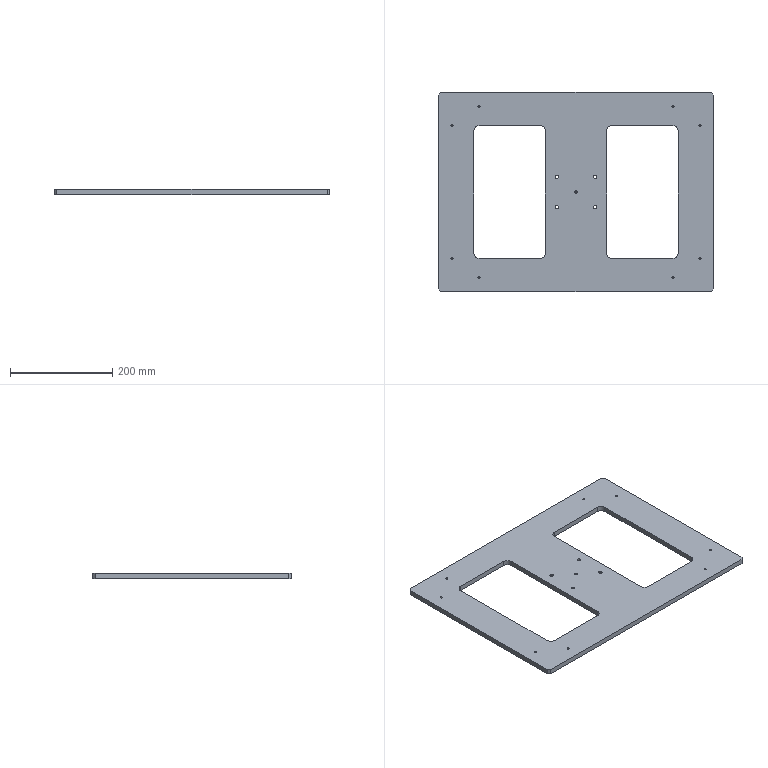Part | 1 solid | 47 faces | box 540 x 390 x 10 mm | volume 1374924 mm3 | cylinder 25 | plane 22 | commonest cylinder face diameters 4.134 x8 20 x8 6.6 x4 11 x4 5 x1
STEP:
#1=CARTESIAN_POINT('',(2.5,0.,0.));
#2=VERTEX_POINT('',#1);
#3=CARTESIAN_POINT('',(0.,0.,0.));
#4=DIRECTION('',(0.,0.,1.));
#5=DIRECTION('',(1.,0.,0.));
#6=AXIS2_PLACEMENT_3D('',#3,#4,#5);
#7=CIRCLE('',#6,2.5);
#8=EDGE_CURVE('',#2,#2,#7,.T.);
#9=ORIENTED_EDGE('',*,*,#8,.T.);
#10=EDGE_LOOP('',(#9));
#11=FACE_BOUND('',#10,.T.);
#12=CARTESIAN_POINT('',(-60.,-120.,0.));
#13=VERTEX_POINT('',#12);
#14=CARTESIAN_POINT('',(-60.,120.,0.));
#15=VERTEX_POINT('',#14);
#16=CARTESIAN_POINT('',(-60.,65.,0.));
#17=DIRECTION('',(0.,1.,0.));
#18=VECTOR('',#17,1000.);
#19=LINE('',#16,#18);
#20=EDGE_CURVE('',#13,#15,#19,.T.);
#21=ORIENTED_EDGE('',*,*,#20,.T.);
#22=CARTESIAN_POINT('',(-70.,130.,0.));
#23=VERTEX_POINT('',#22);
#24=CARTESIAN_POINT('',(-70.,120.,0.));
#25=DIRECTION('',(0.,0.,-1.));
#26=DIRECTION('',(0.7071,0.7071,0.));
#27=AXIS2_PLACEMENT_3D('',#24,#25,#26);
#28=CIRCLE('',#27,10.);
#29=EDGE_CURVE('',#23,#15,#28,.T.);
#30=ORIENTED_EDGE('',*,*,#29,.F.);
#31=CARTESIAN_POINT('',(-190.,130.,0.));
#32=VERTEX_POINT('',#31);
#33=CARTESIAN_POINT('',(-100.,130.,0.));
#34=DIRECTION('',(-1.,0.,0.));
#35=VECTOR('',#34,1000.);
#36=LINE('',#33,#35);
#37=EDGE_CURVE('',#23,#32,#36,.T.);
#38=ORIENTED_EDGE('',*,*,#37,.T.);
#39=CARTESIAN_POINT('',(-200.,120.,0.));
#40=VERTEX_POINT('',#39);
#41=CARTESIAN_POINT('',(-190.,120.,0.));
#42=DIRECTION('',(0.,0.,-1.));
#43=DIRECTION('',(-0.7071,0.7071,0.));
#44=AXIS2_PLACEMENT_3D('',#41,#42,#43);
#45=CIRCLE('',#44,10.);
#46=EDGE_CURVE('',#40,#32,#45,.T.);
#47=ORIENTED_EDGE('',*,*,#46,.F.);
#48=CARTESIAN_POINT('',(-200.,-120.,0.));
#49=VERTEX_POINT('',#48);
#50=CARTESIAN_POINT('',(-200.,-65.,0.));
#51=DIRECTION('',(0.,-1.,0.));
#52=VECTOR('',#51,1000.);
#53=LINE('',#50,#52);
#54=EDGE_CURVE('',#40,#49,#53,.T.);
#55=ORIENTED_EDGE('',*,*,#54,.T.);
#56=CARTESIAN_POINT('',(-190.,-130.,0.));
#57=VERTEX_POINT('',#56);
#58=CARTESIAN_POINT('',(-190.,-120.,0.));
#59=DIRECTION('',(0.,0.,-1.));
#60=DIRECTION('',(-0.7071,-0.7071,0.));
#61=AXIS2_PLACEMENT_3D('',#58,#59,#60);
#62=CIRCLE('',#61,10.);
#63=EDGE_CURVE('',#57,#49,#62,.T.);
#64=ORIENTED_EDGE('',*,*,#63,.F.);
#65=CARTESIAN_POINT('',(-70.,-130.,0.));
#66=VERTEX_POINT('',#65);
#67=CARTESIAN_POINT('',(0.,-130.,0.));
#68=DIRECTION('',(1.,0.,0.));
#69=VECTOR('',#68,1000.);
#70=LINE('',#67,#69);
#71=EDGE_CURVE('',#57,#66,#70,.T.);
#72=ORIENTED_EDGE('',*,*,#71,.T.);
#73=CARTESIAN_POINT('',(-70.,-120.,0.));
#74=DIRECTION('',(0.,0.,-1.));
#75=DIRECTION('',(0.7071,-0.7071,0.));
#76=AXIS2_PLACEMENT_3D('',#73,#74,#75);
#77=CIRCLE('',#76,10.);
#78=EDGE_CURVE('',#13,#66,#77,.T.);
#79=ORIENTED_EDGE('',*,*,#78,.F.);
#80=EDGE_LOOP('',(#21,#30,#38,#47,#55,#64,#72,#79));
#81=FACE_BOUND('',#80,.T.);
#82=CARTESIAN_POINT('',(200.,-120.,0.));
#83=VERTEX_POINT('',#82);
#84=CARTESIAN_POINT('',(200.,120.,0.));
#85=VERTEX_POINT('',#84);
#86=CARTESIAN_POINT('',(200.,65.,0.));
#87=DIRECTION('',(0.,1.,0.));
#88=VECTOR('',#87,1000.);
#89=LINE('',#86,#88);
#90=EDGE_CURVE('',#83,#85,#89,.T.);
#91=ORIENTED_EDGE('',*,*,#90,.T.);
#92=CARTESIAN_POINT('',(190.,130.,0.));
#93=VERTEX_POINT('',#92);
#94=CARTESIAN_POINT('',(190.,120.,0.));
#95=DIRECTION('',(0.,0.,-1.));
#96=DIRECTION('',(0.7071,0.7071,0.));
#97=AXIS2_PLACEMENT_3D('',#94,#95,#96);
#98=CIRCLE('',#97,10.);
#99=EDGE_CURVE('',#93,#85,#98,.T.);
#100=ORIENTED_EDGE('',*,*,#99,.F.);
#101=CARTESIAN_POINT('',(70.,130.,0.));
#102=VERTEX_POINT('',#101);
#103=CARTESIAN_POINT('',(0.,130.,0.));
#104=DIRECTION('',(-1.,0.,0.));
#105=VECTOR('',#104,1000.);
#106=LINE('',#103,#105);
#107=EDGE_CURVE('',#93,#102,#106,.T.);
#108=ORIENTED_EDGE('',*,*,#107,.T.);
#109=CARTESIAN_POINT('',(60.,120.,0.));
#110=VERTEX_POINT('',#109);
#111=CARTESIAN_POINT('',(70.,120.,0.));
#112=DIRECTION('',(0.,0.,-1.));
#113=DIRECTION('',(-0.7071,0.7071,0.));
#114=AXIS2_PLACEMENT_3D('',#111,#112,#113);
#115=CIRCLE('',#114,10.);
#116=EDGE_CURVE('',#110,#102,#115,.T.);
#117=ORIENTED_EDGE('',*,*,#116,.F.);
#118=CARTESIAN_POINT('',(60.,-120.,0.));
#119=VERTEX_POINT('',#118);
#120=CARTESIAN_POINT('',(60.,-65.,0.));
#121=DIRECTION('',(0.,-1.,0.));
#122=VECTOR('',#121,1000.);
#123=LINE('',#120,#122);
#124=EDGE_CURVE('',#110,#119,#123,.T.);
#125=ORIENTED_EDGE('',*,*,#124,.T.);
#126=CARTESIAN_POINT('',(70.,-130.,0.));
#127=VERTEX_POINT('',#126);
#128=CARTESIAN_POINT('',(70.,-120.,0.));
#129=DIRECTION('',(0.,0.,-1.));
#130=DIRECTION('',(-0.7071,-0.7071,0.));
#131=AXIS2_PLACEMENT_3D('',#128,#129,#130);
#132=CIRCLE('',#131,10.);
#133=EDGE_CURVE('',#127,#119,#132,.T.);
#134=ORIENTED_EDGE('',*,*,#133,.F.);
#135=CARTESIAN_POINT('',(190.,-130.,0.));
#136=VERTEX_POINT('',#135);
#137=CARTESIAN_POINT('',(100.,-130.,0.));
#138=DIRECTION('',(1.,0.,0.));
#139=VECTOR('',#138,1000.);
#140=LINE('',#137,#139);
#141=EDGE_CURVE('',#127,#136,#140,.T.);
#142=ORIENTED_EDGE('',*,*,#141,.T.);
#143=CARTESIAN_POINT('',(190.,-120.,0.));
#144=DIRECTION('',(0.,0.,-1.));
#145=DIRECTION('',(0.7071,-0.7071,0.));
#146=AXIS2_PLACEMENT_3D('',#143,#144,#145);
#147=CIRCLE('',#146,10.);
#148=EDGE_CURVE('',#83,#136,#147,.T.);
#149=ORIENTED_EDGE('',*,*,#148,.F.);
#150=EDGE_LOOP('',(#91,#100,#108,#117,#125,#134,#142,#149));
#151=FACE_BOUND('',#150,.T.);
#152=CARTESIAN_POINT('',(-43.,30.,0.));
#153=VERTEX_POINT('',#152);
#154=CARTESIAN_POINT('',(-37.5,30.,0.));
#155=DIRECTION('',(0.,0.,1.));
#156=DIRECTION('',(-1.,0.,0.));
#157=AXIS2_PLACEMENT_3D('',#154,#155,#156);
#158=CIRCLE('',#157,5.5);
#159=EDGE_CURVE('',#153,#153,#158,.T.);
#160=ORIENTED_EDGE('',*,*,#159,.T.);
#161=EDGE_LOOP('',(#160));
#162=FACE_BOUND('',#161,.T.);
#163=CARTESIAN_POINT('',(-43.,-30.,0.));
#164=VERTEX_POINT('',#163);
#165=CARTESIAN_POINT('',(-37.5,-30.,0.));
#166=DIRECTION('',(0.,0.,1.));
#167=DIRECTION('',(-1.,0.,0.));
#168=AXIS2_PLACEMENT_3D('',#165,#166,#167);
#169=CIRCLE('',#168,5.5);
#170=EDGE_CURVE('',#164,#164,#169,.T.);
#171=ORIENTED_EDGE('',*,*,#170,.T.);
#172=EDGE_LOOP('',(#171));
#173=FACE_BOUND('',#172,.T.);
#174=CARTESIAN_POINT('',(32.,-30.,0.));
#175=VERTEX_POINT('',#174);
#176=CARTESIAN_POINT('',(37.5,-30.,0.));
#177=DIRECTION('',(0.,0.,1.));
#178=DIRECTION('',(-1.,0.,0.));
#179=AXIS2_PLACEMENT_3D('',#176,#177,#178);
#180=CIRCLE('',#179,5.5);
#181=EDGE_CURVE('',#175,#175,#180,.T.);
#182=ORIENTED_EDGE('',*,*,#181,.T.);
#183=EDGE_LOOP('',(#182));
#184=FACE_BOUND('',#183,.T.);
#185=CARTESIAN_POINT('',(32.,30.,0.));
#186=VERTEX_POINT('',#185);
#187=CARTESIAN_POINT('',(37.5,30.,0.));
#188=DIRECTION('',(0.,0.,1.));
#189=DIRECTION('',(-1.,0.,0.));
#190=AXIS2_PLACEMENT_3D('',#187,#188,#189);
#191=CIRCLE('',#190,5.5);
#192=EDGE_CURVE('',#186,#186,#191,.T.);
#193=ORIENTED_EDGE('',*,*,#192,.T.);
#194=EDGE_LOOP('',(#193));
#195=FACE_BOUND('',#194,.T.);
#196=CARTESIAN_POINT('',(192.067,168.,0.));
#197=VERTEX_POINT('',#196);
#198=CARTESIAN_POINT('',(190.,168.,0.));
#199=DIRECTION('',(0.,0.,1.));
#200=DIRECTION('',(1.,0.,0.));
#201=AXIS2_PLACEMENT_3D('',#198,#199,#200);
#202=CIRCLE('',#201,2.067);
#203=EDGE_CURVE('',#197,#197,#202,.T.);
#204=ORIENTED_EDGE('',*,*,#203,.T.);
#205=EDGE_LOOP('',(#204));
#206=FACE_BOUND('',#205,.T.);
#207=CARTESIAN_POINT('',(245.067,130.,0.));
#208=VERTEX_POINT('',#207);
#209=CARTESIAN_POINT('',(243.,130.,0.));
#210=DIRECTION('',(0.,0.,1.));
#211=DIRECTION('',(1.,0.,0.));
#212=AXIS2_PLACEMENT_3D('',#209,#210,#211);
#213=CIRCLE('',#212,2.067);
#214=EDGE_CURVE('',#208,#208,#213,.T.);
#215=ORIENTED_EDGE('',*,*,#214,.T.);
#216=EDGE_LOOP('',(#215));
#217=FACE_BOUND('',#216,.T.);
#218=CARTESIAN_POINT('',(-187.933,168.,0.));
#219=VERTEX_POINT('',#218);
#220=CARTESIAN_POINT('',(-190.,168.,0.));
#221=DIRECTION('',(0.,0.,1.));
#222=DIRECTION('',(1.,0.,0.));
#223=AXIS2_PLACEMENT_3D('',#220,#221,#222);
#224=CIRCLE('',#223,2.067);
#225=EDGE_CURVE('',#219,#219,#224,.T.);
#226=ORIENTED_EDGE('',*,*,#225,.T.);
#227=EDGE_LOOP('',(#226));
#228=FACE_BOUND('',#227,.T.);
#229=CARTESIAN_POINT('',(-240.933,130.,0.));
#230=VERTEX_POINT('',#229);
#231=CARTESIAN_POINT('',(-243.,130.,0.));
#232=DIRECTION('',(0.,0.,1.));
#233=DIRECTION('',(1.,0.,0.));
#234=AXIS2_PLACEMENT_3D('',#231,#232,#233);
#235=CIRCLE('',#234,2.067);
#236=EDGE_CURVE('',#230,#230,#235,.T.);
#237=ORIENTED_EDGE('',*,*,#236,.T.);
#238=EDGE_LOOP('',(#237));
#239=FACE_BOUND('',#238,.T.);
#240=CARTESIAN_POINT('',(-240.933,-130.,0.));
#241=VERTEX_POINT('',#240);
#242=CARTESIAN_POINT('',(-243.,-130.,0.));
#243=DIRECTION('',(0.,0.,1.));
#244=DIRECTION('',(1.,0.,0.));
#245=AXIS2_PLACEMENT_3D('',#242,#243,#244);
#246=CIRCLE('',#245,2.067);
#247=EDGE_CURVE('',#241,#241,#246,.T.);
#248=ORIENTED_EDGE('',*,*,#247,.T.);
#249=EDGE_LOOP('',(#248));
#250=FACE_BOUND('',#249,.T.);
#251=CARTESIAN_POINT('',(-187.933,-168.,0.));
#252=VERTEX_POINT('',#251);
#253=CARTESIAN_POINT('',(-190.,-168.,0.));
#254=DIRECTION('',(0.,0.,1.));
#255=DIRECTION('',(1.,0.,0.));
#256=AXIS2_PLACEMENT_3D('',#253,#254,#255);
#257=CIRCLE('',#256,2.067);
#258=EDGE_CURVE('',#252,#252,#257,.T.);
#259=ORIENTED_EDGE('',*,*,#258,.T.);
#260=EDGE_LOOP('',(#259));
#261=FACE_BOUND('',#260,.T.);
#262=CARTESIAN_POINT('',(192.067,-168.,0.));
#263=VERTEX_POINT('',#262);
#264=CARTESIAN_POINT('',(190.,-168.,0.));
#265=DIRECTION('',(0.,0.,1.));
#266=DIRECTION('',(1.,0.,0.));
#267=AXIS2_PLACEMENT_3D('',#264,#265,#266);
#268=CIRCLE('',#267,2.067);
#269=EDGE_CURVE('',#263,#263,#268,.T.);
#270=ORIENTED_EDGE('',*,*,#269,.T.);
#271=EDGE_LOOP('',(#270));
#272=FACE_BOUND('',#271,.T.);
#273=CARTESIAN_POINT('',(245.067,-130.,0.));
#274=VERTEX_POINT('',#273);
#275=CARTESIAN_POINT('',(243.,-130.,0.));
#276=DIRECTION('',(0.,0.,1.));
#277=DIRECTION('',(1.,0.,0.));
#278=AXIS2_PLACEMENT_3D('',#275,#276,#277);
#279=CIRCLE('',#278,2.067);
#280=EDGE_CURVE('',#274,#274,#279,.T.);
#281=ORIENTED_EDGE('',*,*,#280,.T.);
#282=EDGE_LOOP('',(#281));
#283=FACE_BOUND('',#282,.T.);
#284=CARTESIAN_POINT('',(-265.,195.,0.));
#285=VERTEX_POINT('',#284);
#286=CARTESIAN_POINT('',(-270.,190.,0.));
#287=VERTEX_POINT('',#286);
#288=CARTESIAN_POINT('',(-248.75,211.25,0.));
#289=DIRECTION('',(-0.7071,-0.7071,0.));
#290=VECTOR('',#289,1000.);
#291=LINE('',#288,#290);
#292=EDGE_CURVE('',#285,#287,#291,.T.);
#293=ORIENTED_EDGE('',*,*,#292,.F.);
#294=CARTESIAN_POINT('',(265.,195.,0.));
#295=VERTEX_POINT('',#294);
#296=CARTESIAN_POINT('',(270.,195.,0.));
#297=DIRECTION('',(-1.,0.,0.));
#298=VECTOR('',#297,1000.);
#299=LINE('',#296,#298);
#300=EDGE_CURVE('',#295,#285,#299,.T.);
#301=ORIENTED_EDGE('',*,*,#300,.F.);
#302=CARTESIAN_POINT('',(270.,190.,0.));
#303=VERTEX_POINT('',#302);
#304=CARTESIAN_POINT('',(248.75,211.25,0.));
#305=DIRECTION('',(-0.7071,0.7071,0.));
#306=VECTOR('',#305,1000.);
#307=LINE('',#304,#306);
#308=EDGE_CURVE('',#303,#295,#307,.T.);
#309=ORIENTED_EDGE('',*,*,#308,.F.);
#310=CARTESIAN_POINT('',(270.,-190.,0.));
#311=VERTEX_POINT('',#310);
#312=CARTESIAN_POINT('',(270.,-195.,0.));
#313=DIRECTION('',(0.,1.,0.));
#314=VECTOR('',#313,1000.);
#315=LINE('',#312,#314);
#316=EDGE_CURVE('',#311,#303,#315,.T.);
#317=ORIENTED_EDGE('',*,*,#316,.F.);
#318=CARTESIAN_POINT('',(265.,-195.,0.));
#319=VERTEX_POINT('',#318);
#320=CARTESIAN_POINT('',(248.75,-211.25,0.));
#321=DIRECTION('',(0.7071,0.7071,0.));
#322=VECTOR('',#321,1000.);
#323=LINE('',#320,#322);
#324=EDGE_CURVE('',#319,#311,#323,.T.);
#325=ORIENTED_EDGE('',*,*,#324,.F.);
#326=CARTESIAN_POINT('',(-265.,-195.,0.));
#327=VERTEX_POINT('',#326);
#328=CARTESIAN_POINT('',(-270.,-195.,0.));
#329=DIRECTION('',(1.,0.,0.));
#330=VECTOR('',#329,1000.);
#331=LINE('',#328,#330);
#332=EDGE_CURVE('',#327,#319,#331,.T.);
#333=ORIENTED_EDGE('',*,*,#332,.F.);
#334=CARTESIAN_POINT('',(-270.,-190.,0.));
#335=VERTEX_POINT('',#334);
#336=CARTESIAN_POINT('',(-248.75,-211.25,0.));
#337=DIRECTION('',(0.7071,-0.7071,0.));
#338=VECTOR('',#337,1000.);
#339=LINE('',#336,#338);
#340=EDGE_CURVE('',#335,#327,#339,.T.);
#341=ORIENTED_EDGE('',*,*,#340,.F.);
#342=CARTESIAN_POINT('',(-270.,195.,0.));
#343=DIRECTION('',(0.,-1.,0.));
#344=VECTOR('',#343,1000.);
#345=LINE('',#342,#344);
#346=EDGE_CURVE('',#287,#335,#345,.T.);
#347=ORIENTED_EDGE('',*,*,#346,.F.);
#348=EDGE_LOOP('',(#293,#301,#309,#317,#325,#333,#341,#347));
#349=FACE_BOUND('',#348,.T.);
#350=CARTESIAN_POINT('',(0.,0.,0.));
#351=DIRECTION('',(0.,0.,1.));
#352=DIRECTION('',(1.,0.,0.));
#353=AXIS2_PLACEMENT_3D('',#350,#351,#352);
#354=PLANE('',#353);
#355=ADVANCED_FACE('',(#11,#81,#151,#162,#173,#184,#195,#206,#217,#228,#239,#250,#261,#272,#283,#349),#354,.F.);
#356=CARTESIAN_POINT('',(-265.,-195.,10.));
#357=VERTEX_POINT('',#356);
#358=CARTESIAN_POINT('',(-265.,-195.,0.));
#359=DIRECTION('',(0.,0.,1.));
#360=VECTOR('',#359,1000.);
#361=LINE('',#358,#360);
#362=EDGE_CURVE('',#327,#357,#361,.T.);
#363=ORIENTED_EDGE('',*,*,#362,.F.);
#364=ORIENTED_EDGE('',*,*,#332,.T.);
#365=CARTESIAN_POINT('',(265.,-195.,10.));
#366=VERTEX_POINT('',#365);
#367=CARTESIAN_POINT('',(265.,-195.,0.));
#368=DIRECTION('',(0.,0.,-1.));
#369=VECTOR('',#368,1000.);
#370=LINE('',#367,#369);
#371=EDGE_CURVE('',#366,#319,#370,.T.);
#372=ORIENTED_EDGE('',*,*,#371,.F.);
#373=CARTESIAN_POINT('',(-270.,-195.,10.));
#374=DIRECTION('',(1.,0.,0.));
#375=VECTOR('',#374,1000.);
#376=LINE('',#373,#375);
#377=EDGE_CURVE('',#357,#366,#376,.T.);
#378=ORIENTED_EDGE('',*,*,#377,.F.);
#379=EDGE_LOOP('',(#363,#364,#372,#378));
#380=FACE_BOUND('',#379,.T.);
#381=CARTESIAN_POINT('',(-270.,-195.,0.));
#382=DIRECTION('',(0.,-1.,0.));
#383=DIRECTION('',(1.,0.,0.));
#384=AXIS2_PLACEMENT_3D('',#381,#382,#383);
#385=PLANE('',#384);
#386=ADVANCED_FACE('',(#380),#385,.T.);
#387=ORIENTED_EDGE('',*,*,#8,.F.);
#388=EDGE_LOOP('',(#387));
#389=FACE_BOUND('',#388,.T.);
#390=CARTESIAN_POINT('',(2.5,0.,10.));
#391=VERTEX_POINT('',#390);
#392=CARTESIAN_POINT('',(0.,0.,10.));
#393=DIRECTION('',(0.,0.,-1.));
#394=DIRECTION('',(1.,0.,0.));
#395=AXIS2_PLACEMENT_3D('',#392,#393,#394);
#396=CIRCLE('',#395,2.5);
#397=EDGE_CURVE('',#391,#391,#396,.T.);
#398=ORIENTED_EDGE('',*,*,#397,.F.);
#399=EDGE_LOOP('',(#398));
#400=FACE_BOUND('',#399,.T.);
#401=CARTESIAN_POINT('',(0.,0.,-656.183));
#402=DIRECTION('',(0.,0.,1.));
#403=DIRECTION('',(1.,0.,0.));
#404=AXIS2_PLACEMENT_3D('',#401,#402,#403);
#405=CYLINDRICAL_SURFACE('',#404,2.5);
#406=ADVANCED_FACE('',(#389,#400),#405,.F.);
#407=CARTESIAN_POINT('',(-200.,-120.,10.));
#408=VERTEX_POINT('',#407);
#409=CARTESIAN_POINT('',(-200.,-120.,10.));
#410=DIRECTION('',(0.,0.,1.));
#411=VECTOR('',#410,1000.);
#412=LINE('',#409,#411);
#413=EDGE_CURVE('',#49,#408,#412,.T.);
#414=ORIENTED_EDGE('',*,*,#413,.F.);
#415=ORIENTED_EDGE('',*,*,#54,.F.);
#416=CARTESIAN_POINT('',(-200.,120.,10.));
#417=VERTEX_POINT('',#416);
#418=CARTESIAN_POINT('',(-200.,120.,10.));
#419=DIRECTION('',(0.,0.,-1.));
#420=VECTOR('',#419,1000.);
#421=LINE('',#418,#420);
#422=EDGE_CURVE('',#417,#40,#421,.T.);
#423=ORIENTED_EDGE('',*,*,#422,.F.);
#424=CARTESIAN_POINT('',(-200.,-65.,10.));
#425=DIRECTION('',(0.,1.,0.));
#426=VECTOR('',#425,1000.);
#427=LINE('',#424,#426);
#428=EDGE_CURVE('',#408,#417,#427,.T.);
#429=ORIENTED_EDGE('',*,*,#428,.F.);
#430=EDGE_LOOP('',(#414,#415,#423,#429));
#431=FACE_BOUND('',#430,.T.);
#432=CARTESIAN_POINT('',(-200.,-130.,10.));
#433=DIRECTION('',(-1.,0.,0.));
#434=DIRECTION('',(0.,1.,0.));
#435=AXIS2_PLACEMENT_3D('',#432,#433,#434);
#436=PLANE('',#435);
#437=ADVANCED_FACE('',(#431),#436,.F.);
#438=CARTESIAN_POINT('',(-190.,130.,10.));
#439=VERTEX_POINT('',#438);
#440=CARTESIAN_POINT('',(-190.,120.,10.));
#441=DIRECTION('',(0.,0.,1.));
#442=DIRECTION('',(-0.7071,0.7071,0.));
#443=AXIS2_PLACEMENT_3D('',#440,#441,#442);
#444=CIRCLE('',#443,10.);
#445=EDGE_CURVE('',#439,#417,#444,.T.);
#446=ORIENTED_EDGE('',*,*,#445,.T.);
#447=ORIENTED_EDGE('',*,*,#422,.T.);
#448=ORIENTED_EDGE('',*,*,#46,.T.);
#449=CARTESIAN_POINT('',(-190.,130.,10.));
#450=DIRECTION('',(0.,0.,1.));
#451=VECTOR('',#450,1000.);
#452=LINE('',#449,#451);
#453=EDGE_CURVE('',#32,#439,#452,.T.);
#454=ORIENTED_EDGE('',*,*,#453,.T.);
#455=EDGE_LOOP('',(#446,#447,#448,#454));
#456=FACE_BOUND('',#455,.T.);
#457=CARTESIAN_POINT('',(-190.,120.,10.));
#458=DIRECTION('',(0.,0.,-1.));
#459=DIRECTION('',(-0.7071,0.7071,0.));
#460=AXIS2_PLACEMENT_3D('',#457,#458,#459);
#461=CYLINDRICAL_SURFACE('',#460,10.);
#462=ADVANCED_FACE('',(#456),#461,.F.);
#463=CARTESIAN_POINT('',(-70.,130.,10.));
#464=VERTEX_POINT('',#463);
#465=CARTESIAN_POINT('',(-70.,130.,10.));
#466=DIRECTION('',(0.,0.,-1.));
#467=VECTOR('',#466,1000.);
#468=LINE('',#465,#467);
#469=EDGE_CURVE('',#464,#23,#468,.T.);
#470=ORIENTED_EDGE('',*,*,#469,.F.);
#471=CARTESIAN_POINT('',(-100.,130.,10.));
#472=DIRECTION('',(1.,0.,0.));
#473=VECTOR('',#472,1000.);
#474=LINE('',#471,#473);
#475=EDGE_CURVE('',#439,#464,#474,.T.);
#476=ORIENTED_EDGE('',*,*,#475,.F.);
#477=ORIENTED_EDGE('',*,*,#453,.F.);
#478=ORIENTED_EDGE('',*,*,#37,.F.);
#479=EDGE_LOOP('',(#470,#476,#477,#478));
#480=FACE_BOUND('',#479,.T.);
#481=CARTESIAN_POINT('',(-200.,130.,10.));
#482=DIRECTION('',(0.,1.,0.));
#483=DIRECTION('',(1.,0.,0.));
#484=AXIS2_PLACEMENT_3D('',#481,#482,#483);
#485=PLANE('',#484);
#486=ADVANCED_FACE('',(#480),#485,.F.);
#487=CARTESIAN_POINT('',(-60.,120.,10.));
#488=VERTEX_POINT('',#487);
#489=CARTESIAN_POINT('',(-70.,120.,10.));
#490=DIRECTION('',(0.,0.,1.));
#491=DIRECTION('',(0.7071,0.7071,0.));
#492=AXIS2_PLACEMENT_3D('',#489,#490,#491);
#493=CIRCLE('',#492,10.);
#494=EDGE_CURVE('',#488,#464,#493,.T.);
#495=ORIENTED_EDGE('',*,*,#494,.T.);
#496=ORIENTED_EDGE('',*,*,#469,.T.);
#497=ORIENTED_EDGE('',*,*,#29,.T.);
#498=CARTESIAN_POINT('',(-60.,120.,10.));
#499=DIRECTION('',(0.,0.,1.));
#500=VECTOR('',#499,1000.);
#501=LINE('',#498,#500);
#502=EDGE_CURVE('',#15,#488,#501,.T.);
#503=ORIENTED_EDGE('',*,*,#502,.T.);
#504=EDGE_LOOP('',(#495,#496,#497,#503));
#505=FACE_BOUND('',#504,.T.);
#506=CARTESIAN_POINT('',(-70.,120.,10.));
#507=DIRECTION('',(0.,0.,-1.));
#508=DIRECTION('',(0.7071,0.7071,0.));
#509=AXIS2_PLACEMENT_3D('',#506,#507,#508);
#510=CYLINDRICAL_SURFACE('',#509,10.);
#511=ADVANCED_FACE('',(#505),#510,.F.);
#512=CARTESIAN_POINT('',(-70.,-130.,10.));
#513=VERTEX_POINT('',#512);
#514=CARTESIAN_POINT('',(-70.,-130.,10.));
#515=DIRECTION('',(0.,0.,1.));
#516=VECTOR('',#515,1000.);
#517=LINE('',#514,#516);
#518=EDGE_CURVE('',#66,#513,#517,.T.);
#519=ORIENTED_EDGE('',*,*,#518,.F.);
#520=ORIENTED_EDGE('',*,*,#71,.F.);
#521=CARTESIAN_POINT('',(-190.,-130.,10.));
#522=VERTEX_POINT('',#521);
#523=CARTESIAN_POINT('',(-190.,-130.,10.));
#524=DIRECTION('',(0.,0.,-1.));
#525=VECTOR('',#524,1000.);
#526=LINE('',#523,#525);
#527=EDGE_CURVE('',#522,#57,#526,.T.);
#528=ORIENTED_EDGE('',*,*,#527,.F.);
#529=CARTESIAN_POINT('',(0.,-130.,10.));
#530=DIRECTION('',(-1.,0.,0.));
#531=VECTOR('',#530,1000.);
#532=LINE('',#529,#531);
#533=EDGE_CURVE('',#513,#522,#532,.T.);
#534=ORIENTED_EDGE('',*,*,#533,.F.);
#535=EDGE_LOOP('',(#519,#520,#528,#534));
#536=FACE_BOUND('',#535,.T.);
#537=CARTESIAN_POINT('',(200.,-130.,10.));
#538=DIRECTION('',(0.,-1.,0.));
#539=DIRECTION('',(-1.,0.,0.));
#540=AXIS2_PLACEMENT_3D('',#537,#538,#539);
#541=PLANE('',#540);
#542=ADVANCED_FACE('',(#536),#541,.F.);
#543=CARTESIAN_POINT('',(-190.,-120.,10.));
#544=DIRECTION('',(0.,0.,1.));
#545=DIRECTION('',(-0.7071,-0.7071,0.));
#546=AXIS2_PLACEMENT_3D('',#543,#544,#545);
#547=CIRCLE('',#546,10.);
#548=EDGE_CURVE('',#408,#522,#547,.T.);
#549=ORIENTED_EDGE('',*,*,#548,.T.);
#550=ORIENTED_EDGE('',*,*,#527,.T.);
#551=ORIENTED_EDGE('',*,*,#63,.T.);
#552=ORIENTED_EDGE('',*,*,#413,.T.);
#553=EDGE_LOOP('',(#549,#550,#551,#552));
#554=FACE_BOUND('',#553,.T.);
#555=CARTESIAN_POINT('',(-190.,-120.,10.));
#556=DIRECTION('',(0.,0.,-1.));
#557=DIRECTION('',(-0.7071,-0.7071,0.));
#558=AXIS2_PLACEMENT_3D('',#555,#556,#557);
#559=CYLINDRICAL_SURFACE('',#558,10.);
#560=ADVANCED_FACE('',(#554),#559,.F.);
#561=CARTESIAN_POINT('',(-60.,-120.,10.));
#562=VERTEX_POINT('',#561);
#563=CARTESIAN_POINT('',(-60.,-120.,10.));
#564=DIRECTION('',(0.,0.,-1.));
#565=VECTOR('',#564,1000.);
#566=LINE('',#563,#565);
#567=EDGE_CURVE('',#562,#13,#566,.T.);
#568=ORIENTED_EDGE('',*,*,#567,.F.);
#569=CARTESIAN_POINT('',(-60.,65.,10.));
#570=DIRECTION('',(0.,-1.,0.));
#571=VECTOR('',#570,1000.);
#572=LINE('',#569,#571);
#573=EDGE_CURVE('',#488,#562,#572,.T.);
#574=ORIENTED_EDGE('',*,*,#573,.F.);
#575=ORIENTED_EDGE('',*,*,#502,.F.);
#576=ORIENTED_EDGE('',*,*,#20,.F.);
#577=EDGE_LOOP('',(#568,#574,#575,#576));
#578=FACE_BOUND('',#577,.T.);
#579=CARTESIAN_POINT('',(-60.,130.,10.));
#580=DIRECTION('',(1.,0.,0.));
#581=DIRECTION('',(0.,-1.,0.));
#582=AXIS2_PLACEMENT_3D('',#579,#580,#581);
#583=PLANE('',#582);
#584=ADVANCED_FACE('',(#578),#583,.F.);
#585=CARTESIAN_POINT('',(-70.,-120.,10.));
#586=DIRECTION('',(0.,0.,1.));
#587=DIRECTION('',(0.7071,-0.7071,0.));
#588=AXIS2_PLACEMENT_3D('',#585,#586,#587);
#589=CIRCLE('',#588,10.);
#590=EDGE_CURVE('',#513,#562,#589,.T.);
#591=ORIENTED_EDGE('',*,*,#590,.T.);
#592=ORIENTED_EDGE('',*,*,#567,.T.);
#593=ORIENTED_EDGE('',*,*,#78,.T.);
#594=ORIENTED_EDGE('',*,*,#518,.T.);
#595=EDGE_LOOP('',(#591,#592,#593,#594));
#596=FACE_BOUND('',#595,.T.);
#597=CARTESIAN_POINT('',(-70.,-120.,10.));
#598=DIRECTION('',(0.,0.,-1.));
#599=DIRECTION('',(0.7071,-0.7071,0.));
#600=AXIS2_PLACEMENT_3D('',#597,#598,#599);
#601=CYLINDRICAL_SURFACE('',#600,10.);
#602=ADVANCED_FACE('',(#596),#601,.F.);
#603=CARTESIAN_POINT('',(190.,-130.,10.));
#604=VERTEX_POINT('',#603);
#605=CARTESIAN_POINT('',(190.,-130.,10.));
#606=DIRECTION('',(0.,0.,1.));
#607=VECTOR('',#606,1000.);
#608=LINE('',#605,#607);
#609=EDGE_CURVE('',#136,#604,#608,.T.);
#610=ORIENTED_EDGE('',*,*,#609,.F.);
#611=ORIENTED_EDGE('',*,*,#141,.F.);
#612=CARTESIAN_POINT('',(70.,-130.,10.));
#613=VERTEX_POINT('',#612);
#614=CARTESIAN_POINT('',(70.,-130.,10.));
#615=DIRECTION('',(0.,0.,-1.));
#616=VECTOR('',#615,1000.);
#617=LINE('',#614,#616);
#618=EDGE_CURVE('',#613,#127,#617,.T.);
#619=ORIENTED_EDGE('',*,*,#618,.F.);
#620=CARTESIAN_POINT('',(100.,-130.,10.));
#621=DIRECTION('',(-1.,0.,0.));
#622=VECTOR('',#621,1000.);
#623=LINE('',#620,#622);
#624=EDGE_CURVE('',#604,#613,#623,.T.);
#625=ORIENTED_EDGE('',*,*,#624,.F.);
#626=EDGE_LOOP('',(#610,#611,#619,#625));
#627=FACE_BOUND('',#626,.T.);
#628=CARTESIAN_POINT('',(200.,-130.,10.));
#629=DIRECTION('',(0.,-1.,0.));
#630=DIRECTION('',(-1.,0.,0.));
#631=AXIS2_PLACEMENT_3D('',#628,#629,#630);
#632=PLANE('',#631);
#633=ADVANCED_FACE('',(#627),#632,.F.);
#634=CARTESIAN_POINT('',(60.,-120.,10.));
#635=VERTEX_POINT('',#634);
#636=CARTESIAN_POINT('',(70.,-120.,10.));
#637=DIRECTION('',(0.,0.,1.));
#638=DIRECTION('',(-0.7071,-0.7071,0.));
#639=AXIS2_PLACEMENT_3D('',#636,#637,#638);
#640=CIRCLE('',#639,10.);
#641=EDGE_CURVE('',#635,#613,#640,.T.);
#642=ORIENTED_EDGE('',*,*,#641,.T.);
#643=ORIENTED_EDGE('',*,*,#618,.T.);
#644=ORIENTED_EDGE('',*,*,#133,.T.);
#645=CARTESIAN_POINT('',(60.,-120.,10.));
#646=DIRECTION('',(0.,0.,1.));
#647=VECTOR('',#646,1000.);
#648=LINE('',#645,#647);
#649=EDGE_CURVE('',#119,#635,#648,.T.);
#650=ORIENTED_EDGE('',*,*,#649,.T.);
#651=EDGE_LOOP('',(#642,#643,#644,#650));
#652=FACE_BOUND('',#651,.T.);
#653=CARTESIAN_POINT('',(70.,-120.,10.));
#654=DIRECTION('',(0.,0.,-1.));
#655=DIRECTION('',(-0.7071,-0.7071,0.));
#656=AXIS2_PLACEMENT_3D('',#653,#654,#655);
#657=CYLINDRICAL_SURFACE('',#656,10.);
#658=ADVANCED_FACE('',(#652),#657,.F.);
#659=CARTESIAN_POINT('',(200.,120.,10.));
#660=VERTEX_POINT('',#659);
#661=CARTESIAN_POINT('',(200.,120.,10.));
#662=DIRECTION('',(0.,0.,1.));
#663=VECTOR('',#662,1000.);
#664=LINE('',#661,#663);
#665=EDGE_CURVE('',#85,#660,#664,.T.);
#666=ORIENTED_EDGE('',*,*,#665,.F.);
#667=ORIENTED_EDGE('',*,*,#90,.F.);
#668=CARTESIAN_POINT('',(200.,-120.,10.));
#669=VERTEX_POINT('',#668);
#670=CARTESIAN_POINT('',(200.,-120.,10.));
#671=DIRECTION('',(0.,0.,-1.));
#672=VECTOR('',#671,1000.);
#673=LINE('',#670,#672);
#674=EDGE_CURVE('',#669,#83,#673,.T.);
#675=ORIENTED_EDGE('',*,*,#674,.F.);
#676=CARTESIAN_POINT('',(200.,65.,10.));
#677=DIRECTION('',(0.,-1.,0.));
#678=VECTOR('',#677,1000.);
#679=LINE('',#676,#678);
#680=EDGE_CURVE('',#660,#669,#679,.T.);
#681=ORIENTED_EDGE('',*,*,#680,.F.);
#682=EDGE_LOOP('',(#666,#667,#675,#681));
#683=FACE_BOUND('',#682,.T.);
#684=CARTESIAN_POINT('',(200.,130.,10.));
#685=DIRECTION('',(1.,0.,0.));
#686=DIRECTION('',(0.,-1.,0.));
#687=AXIS2_PLACEMENT_3D('',#684,#685,#686);
#688=PLANE('',#687);
#689=ADVANCED_FACE('',(#683),#688,.F.);
#690=CARTESIAN_POINT('',(190.,-120.,10.));
#691=DIRECTION('',(0.,0.,1.));
#692=DIRECTION('',(0.7071,-0.7071,0.));
#693=AXIS2_PLACEMENT_3D('',#690,#691,#692);
#694=CIRCLE('',#693,10.);
#695=EDGE_CURVE('',#604,#669,#694,.T.);
#696=ORIENTED_EDGE('',*,*,#695,.T.);
#697=ORIENTED_EDGE('',*,*,#674,.T.);
#698=ORIENTED_EDGE('',*,*,#148,.T.);
#699=ORIENTED_EDGE('',*,*,#609,.T.);
#700=EDGE_LOOP('',(#696,#697,#698,#699));
#701=FACE_BOUND('',#700,.T.);
#702=CARTESIAN_POINT('',(190.,-120.,10.));
#703=DIRECTION('',(0.,0.,-1.));
#704=DIRECTION('',(0.7071,-0.7071,0.));
#705=AXIS2_PLACEMENT_3D('',#702,#703,#704);
#706=CYLINDRICAL_SURFACE('',#705,10.);
#707=ADVANCED_FACE('',(#701),#706,.F.);
#708=CARTESIAN_POINT('',(60.,120.,10.));
#709=VERTEX_POINT('',#708);
#710=CARTESIAN_POINT('',(60.,120.,10.));
#711=DIRECTION('',(0.,0.,-1.));
#712=VECTOR('',#711,1000.);
#713=LINE('',#710,#712);
#714=EDGE_CURVE('',#709,#110,#713,.T.);
#715=ORIENTED_EDGE('',*,*,#714,.F.);
#716=CARTESIAN_POINT('',(60.,-65.,10.));
#717=DIRECTION('',(0.,1.,0.));
#718=VECTOR('',#717,1000.);
#719=LINE('',#716,#718);
#720=EDGE_CURVE('',#635,#709,#719,.T.);
#721=ORIENTED_EDGE('',*,*,#720,.F.);
#722=ORIENTED_EDGE('',*,*,#649,.F.);
#723=ORIENTED_EDGE('',*,*,#124,.F.);
#724=EDGE_LOOP('',(#715,#721,#722,#723));
#725=FACE_BOUND('',#724,.T.);
#726=CARTESIAN_POINT('',(60.,-130.,10.));
#727=DIRECTION('',(-1.,0.,0.));
#728=DIRECTION('',(0.,1.,0.));
#729=AXIS2_PLACEMENT_3D('',#726,#727,#728);
#730=PLANE('',#729);
#731=ADVANCED_FACE('',(#725),#730,.F.);
#732=CARTESIAN_POINT('',(70.,130.,10.));
#733=VERTEX_POINT('',#732);
#734=CARTESIAN_POINT('',(70.,120.,10.));
#735=DIRECTION('',(0.,0.,1.));
#736=DIRECTION('',(-0.7071,0.7071,0.));
#737=AXIS2_PLACEMENT_3D('',#734,#735,#736);
#738=CIRCLE('',#737,10.);
#739=EDGE_CURVE('',#733,#709,#738,.T.);
#740=ORIENTED_EDGE('',*,*,#739,.T.);
#741=ORIENTED_EDGE('',*,*,#714,.T.);
#742=ORIENTED_EDGE('',*,*,#116,.T.);
#743=CARTESIAN_POINT('',(70.,130.,10.));
#744=DIRECTION('',(0.,0.,1.));
#745=VECTOR('',#744,1000.);
#746=LINE('',#743,#745);
#747=EDGE_CURVE('',#102,#733,#746,.T.);
#748=ORIENTED_EDGE('',*,*,#747,.T.);
#749=EDGE_LOOP('',(#740,#741,#742,#748));
#750=FACE_BOUND('',#749,.T.);
#751=CARTESIAN_POINT('',(70.,120.,10.));
#752=DIRECTION('',(0.,0.,-1.));
#753=DIRECTION('',(-0.7071,0.7071,0.));
#754=AXIS2_PLACEMENT_3D('',#751,#752,#753);
#755=CYLINDRICAL_SURFACE('',#754,10.);
#756=ADVANCED_FACE('',(#750),#755,.F.);
#757=CARTESIAN_POINT('',(190.,130.,10.));
#758=VERTEX_POINT('',#757);
#759=CARTESIAN_POINT('',(190.,130.,10.));
#760=DIRECTION('',(0.,0.,-1.));
#761=VECTOR('',#760,1000.);
#762=LINE('',#759,#761);
#763=EDGE_CURVE('',#758,#93,#762,.T.);
#764=ORIENTED_EDGE('',*,*,#763,.F.);
#765=CARTESIAN_POINT('',(0.,130.,10.));
#766=DIRECTION('',(1.,0.,0.));
#767=VECTOR('',#766,1000.);
#768=LINE('',#765,#767);
#769=EDGE_CURVE('',#733,#758,#768,.T.);
#770=ORIENTED_EDGE('',*,*,#769,.F.);
#771=ORIENTED_EDGE('',*,*,#747,.F.);
#772=ORIENTED_EDGE('',*,*,#107,.F.);
#773=EDGE_LOOP('',(#764,#770,#771,#772));
#774=FACE_BOUND('',#773,.T.);
#775=CARTESIAN_POINT('',(-200.,130.,10.));
#776=DIRECTION('',(0.,1.,0.));
#777=DIRECTION('',(1.,0.,0.));
#778=AXIS2_PLACEMENT_3D('',#775,#776,#777);
#779=PLANE('',#778);
#780=ADVANCED_FACE('',(#774),#779,.F.);
#781=CARTESIAN_POINT('',(190.,120.,10.));
#782=DIRECTION('',(0.,0.,1.));
#783=DIRECTION('',(0.7071,0.7071,0.));
#784=AXIS2_PLACEMENT_3D('',#781,#782,#783);
#785=CIRCLE('',#784,10.);
#786=EDGE_CURVE('',#660,#758,#785,.T.);
#787=ORIENTED_EDGE('',*,*,#786,.T.);
#788=ORIENTED_EDGE('',*,*,#763,.T.);
#789=ORIENTED_EDGE('',*,*,#99,.T.);
#790=ORIENTED_EDGE('',*,*,#665,.T.);
#791=EDGE_LOOP('',(#787,#788,#789,#790));
#792=FACE_BOUND('',#791,.T.);
#793=CARTESIAN_POINT('',(190.,120.,10.));
#794=DIRECTION('',(0.,0.,-1.));
#795=DIRECTION('',(0.7071,0.7071,0.));
#796=AXIS2_PLACEMENT_3D('',#793,#794,#795);
#797=CYLINDRICAL_SURFACE('',#796,10.);
#798=ADVANCED_FACE('',(#792),#797,.F.);
#799=CARTESIAN_POINT('',(-40.8,30.,10.));
#800=VERTEX_POINT('',#799);
#801=CARTESIAN_POINT('',(-37.5,30.,10.));
#802=DIRECTION('',(0.,0.,-1.));
#803=DIRECTION('',(-1.,0.,0.));
#804=AXIS2_PLACEMENT_3D('',#801,#802,#803);
#805=CIRCLE('',#804,3.3);
#806=EDGE_CURVE('',#800,#800,#805,.T.);
#807=ORIENTED_EDGE('',*,*,#806,.F.);
#808=EDGE_LOOP('',(#807));
#809=FACE_BOUND('',#808,.T.);
#810=CARTESIAN_POINT('',(-40.8,30.,6.8));
#811=VERTEX_POINT('',#810);
#812=CARTESIAN_POINT('',(-37.5,30.,6.8));
#813=DIRECTION('',(0.,0.,-1.));
#814=DIRECTION('',(-1.,0.,0.));
#815=AXIS2_PLACEMENT_3D('',#812,#813,#814);
#816=CIRCLE('',#815,3.3);
#817=EDGE_CURVE('',#811,#811,#816,.T.);
#818=ORIENTED_EDGE('',*,*,#817,.T.);
#819=EDGE_LOOP('',(#818));
#820=FACE_BOUND('',#819,.T.);
#821=CARTESIAN_POINT('',(-37.5,30.,666.183));
#822=DIRECTION('',(0.,0.,-1.));
#823=DIRECTION('',(-1.,0.,0.));
#824=AXIS2_PLACEMENT_3D('',#821,#822,#823);
#825=CYLINDRICAL_SURFACE('',#824,3.3);
#826=ADVANCED_FACE('',(#809,#820),#825,.F.);
#827=CARTESIAN_POINT('',(-43.,30.,6.8));
#828=VERTEX_POINT('',#827);
#829=CARTESIAN_POINT('',(-37.5,30.,6.8));
#830=DIRECTION('',(0.,0.,-1.));
#831=DIRECTION('',(-1.,0.,0.));
#832=AXIS2_PLACEMENT_3D('',#829,#830,#831);
#833=CIRCLE('',#832,5.5);
#834=EDGE_CURVE('',#828,#828,#833,.T.);
#835=ORIENTED_EDGE('',*,*,#834,.F.);
#836=EDGE_LOOP('',(#835));
#837=FACE_BOUND('',#836,.T.);
#838=ORIENTED_EDGE('',*,*,#159,.F.);
#839=EDGE_LOOP('',(#838));
#840=FACE_BOUND('',#839,.T.);
#841=CARTESIAN_POINT('',(-37.5,30.,3.4));
#842=DIRECTION('',(0.,0.,-1.));
#843=DIRECTION('',(-1.,0.,0.));
#844=AXIS2_PLACEMENT_3D('',#841,#842,#843);
#845=CYLINDRICAL_SURFACE('',#844,5.5);
#846=ADVANCED_FACE('',(#837,#840),#845,.F.);
#847=ORIENTED_EDGE('',*,*,#817,.F.);
#848=EDGE_LOOP('',(#847));
#849=FACE_BOUND('',#848,.T.);
#850=ORIENTED_EDGE('',*,*,#834,.T.);
#851=EDGE_LOOP('',(#850));
#852=FACE_BOUND('',#851,.T.);
#853=CARTESIAN_POINT('',(37.5,30.,6.8));
#854=DIRECTION('',(0.,0.,-1.));
#855=DIRECTION('',(-1.,0.,0.));
#856=AXIS2_PLACEMENT_3D('',#853,#854,#855);
#857=PLANE('',#856);
#858=ADVANCED_FACE('',(#849,#852),#857,.T.);
#859=CARTESIAN_POINT('',(-40.8,-30.,10.));
#860=VERTEX_POINT('',#859);
#861=CARTESIAN_POINT('',(-37.5,-30.,10.));
#862=DIRECTION('',(0.,0.,-1.));
#863=DIRECTION('',(-1.,0.,0.));
#864=AXIS2_PLACEMENT_3D('',#861,#862,#863);
#865=CIRCLE('',#864,3.3);
#866=EDGE_CURVE('',#860,#860,#865,.T.);
#867=ORIENTED_EDGE('',*,*,#866,.F.);
#868=EDGE_LOOP('',(#867));
#869=FACE_BOUND('',#868,.T.);
#870=CARTESIAN_POINT('',(-40.8,-30.,6.8));
#871=VERTEX_POINT('',#870);
#872=CARTESIAN_POINT('',(-37.5,-30.,6.8));
#873=DIRECTION('',(0.,0.,-1.));
#874=DIRECTION('',(-1.,0.,0.));
#875=AXIS2_PLACEMENT_3D('',#872,#873,#874);
#876=CIRCLE('',#875,3.3);
#877=EDGE_CURVE('',#871,#871,#876,.T.);
#878=ORIENTED_EDGE('',*,*,#877,.T.);
#879=EDGE_LOOP('',(#878));
#880=FACE_BOUND('',#879,.T.);
#881=CARTESIAN_POINT('',(-37.5,-30.,666.183));
#882=DIRECTION('',(0.,0.,-1.));
#883=DIRECTION('',(-1.,0.,0.));
#884=AXIS2_PLACEMENT_3D('',#881,#882,#883);
#885=CYLINDRICAL_SURFACE('',#884,3.3);
#886=ADVANCED_FACE('',(#869,#880),#885,.F.);
#887=CARTESIAN_POINT('',(-43.,-30.,6.8));
#888=VERTEX_POINT('',#887);
#889=CARTESIAN_POINT('',(-37.5,-30.,6.8));
#890=DIRECTION('',(0.,0.,-1.));
#891=DIRECTION('',(-1.,0.,0.));
#892=AXIS2_PLACEMENT_3D('',#889,#890,#891);
#893=CIRCLE('',#892,5.5);
#894=EDGE_CURVE('',#888,#888,#893,.T.);
#895=ORIENTED_EDGE('',*,*,#894,.F.);
#896=EDGE_LOOP('',(#895));
#897=FACE_BOUND('',#896,.T.);
#898=ORIENTED_EDGE('',*,*,#170,.F.);
#899=EDGE_LOOP('',(#898));
#900=FACE_BOUND('',#899,.T.);
#901=CARTESIAN_POINT('',(-37.5,-30.,3.4));
#902=DIRECTION('',(0.,0.,-1.));
#903=DIRECTION('',(-1.,0.,0.));
#904=AXIS2_PLACEMENT_3D('',#901,#902,#903);
#905=CYLINDRICAL_SURFACE('',#904,5.5);
#906=ADVANCED_FACE('',(#897,#900),#905,.F.);
#907=ORIENTED_EDGE('',*,*,#877,.F.);
#908=EDGE_LOOP('',(#907));
#909=FACE_BOUND('',#908,.T.);
#910=ORIENTED_EDGE('',*,*,#894,.T.);
#911=EDGE_LOOP('',(#910));
#912=FACE_BOUND('',#911,.T.);
#913=CARTESIAN_POINT('',(37.5,30.,6.8));
#914=DIRECTION('',(0.,0.,-1.));
#915=DIRECTION('',(-1.,0.,0.));
#916=AXIS2_PLACEMENT_3D('',#913,#914,#915);
#917=PLANE('',#916);
#918=ADVANCED_FACE('',(#909,#912),#917,.T.);
#919=CARTESIAN_POINT('',(34.2,-30.,10.));
#920=VERTEX_POINT('',#919);
#921=CARTESIAN_POINT('',(37.5,-30.,10.));
#922=DIRECTION('',(0.,0.,-1.));
#923=DIRECTION('',(-1.,0.,0.));
#924=AXIS2_PLACEMENT_3D('',#921,#922,#923);
#925=CIRCLE('',#924,3.3);
#926=EDGE_CURVE('',#920,#920,#925,.T.);
#927=ORIENTED_EDGE('',*,*,#926,.F.);
#928=EDGE_LOOP('',(#927));
#929=FACE_BOUND('',#928,.T.);
#930=CARTESIAN_POINT('',(34.2,-30.,6.8));
#931=VERTEX_POINT('',#930);
#932=CARTESIAN_POINT('',(37.5,-30.,6.8));
#933=DIRECTION('',(0.,0.,-1.));
#934=DIRECTION('',(-1.,0.,0.));
#935=AXIS2_PLACEMENT_3D('',#932,#933,#934);
#936=CIRCLE('',#935,3.3);
#937=EDGE_CURVE('',#931,#931,#936,.T.);
#938=ORIENTED_EDGE('',*,*,#937,.T.);
#939=EDGE_LOOP('',(#938));
#940=FACE_BOUND('',#939,.T.);
#941=CARTESIAN_POINT('',(37.5,-30.,666.183));
#942=DIRECTION('',(0.,0.,-1.));
#943=DIRECTION('',(-1.,0.,0.));
#944=AXIS2_PLACEMENT_3D('',#941,#942,#943);
#945=CYLINDRICAL_SURFACE('',#944,3.3);
#946=ADVANCED_FACE('',(#929,#940),#945,.F.);
#947=CARTESIAN_POINT('',(32.,-30.,6.8));
#948=VERTEX_POINT('',#947);
#949=CARTESIAN_POINT('',(37.5,-30.,6.8));
#950=DIRECTION('',(0.,0.,-1.));
#951=DIRECTION('',(-1.,0.,0.));
#952=AXIS2_PLACEMENT_3D('',#949,#950,#951);
#953=CIRCLE('',#952,5.5);
#954=EDGE_CURVE('',#948,#948,#953,.T.);
#955=ORIENTED_EDGE('',*,*,#954,.F.);
#956=EDGE_LOOP('',(#955));
#957=FACE_BOUND('',#956,.T.);
#958=ORIENTED_EDGE('',*,*,#181,.F.);
#959=EDGE_LOOP('',(#958));
#960=FACE_BOUND('',#959,.T.);
#961=CARTESIAN_POINT('',(37.5,-30.,3.4));
#962=DIRECTION('',(0.,0.,-1.));
#963=DIRECTION('',(-1.,0.,0.));
#964=AXIS2_PLACEMENT_3D('',#961,#962,#963);
#965=CYLINDRICAL_SURFACE('',#964,5.5);
#966=ADVANCED_FACE('',(#957,#960),#965,.F.);
#967=ORIENTED_EDGE('',*,*,#937,.F.);
#968=EDGE_LOOP('',(#967));
#969=FACE_BOUND('',#968,.T.);
#970=ORIENTED_EDGE('',*,*,#954,.T.);
#971=EDGE_LOOP('',(#970));
#972=FACE_BOUND('',#971,.T.);
#973=CARTESIAN_POINT('',(37.5,30.,6.8));
#974=DIRECTION('',(0.,0.,-1.));
#975=DIRECTION('',(-1.,0.,0.));
#976=AXIS2_PLACEMENT_3D('',#973,#974,#975);
#977=PLANE('',#976);
#978=ADVANCED_FACE('',(#969,#972),#977,.T.);
#979=CARTESIAN_POINT('',(34.2,30.,10.));
#980=VERTEX_POINT('',#979);
#981=CARTESIAN_POINT('',(37.5,30.,10.));
#982=DIRECTION('',(0.,0.,-1.));
#983=DIRECTION('',(-1.,0.,0.));
#984=AXIS2_PLACEMENT_3D('',#981,#982,#983);
#985=CIRCLE('',#984,3.3);
#986=EDGE_CURVE('',#980,#980,#985,.T.);
#987=ORIENTED_EDGE('',*,*,#986,.F.);
#988=EDGE_LOOP('',(#987));
#989=FACE_BOUND('',#988,.T.);
#990=CARTESIAN_POINT('',(34.2,30.,6.8));
#991=VERTEX_POINT('',#990);
#992=CARTESIAN_POINT('',(37.5,30.,6.8));
#993=DIRECTION('',(0.,0.,-1.));
#994=DIRECTION('',(-1.,0.,0.));
#995=AXIS2_PLACEMENT_3D('',#992,#993,#994);
#996=CIRCLE('',#995,3.3);
#997=EDGE_CURVE('',#991,#991,#996,.T.);
#998=ORIENTED_EDGE('',*,*,#997,.T.);
#999=EDGE_LOOP('',(#998));
#1000=FACE_BOUND('',#999,.T.);
#1001=CARTESIAN_POINT('',(37.5,30.,666.183));
#1002=DIRECTION('',(0.,0.,-1.));
#1003=DIRECTION('',(-1.,0.,0.));
#1004=AXIS2_PLACEMENT_3D('',#1001,#1002,#1003);
#1005=CYLINDRICAL_SURFACE('',#1004,3.3);
#1006=ADVANCED_FACE('',(#989,#1000),#1005,.F.);
#1007=CARTESIAN_POINT('',(32.,30.,6.8));
#1008=VERTEX_POINT('',#1007);
#1009=CARTESIAN_POINT('',(37.5,30.,6.8));
#1010=DIRECTION('',(0.,0.,-1.));
#1011=DIRECTION('',(-1.,0.,0.));
#1012=AXIS2_PLACEMENT_3D('',#1009,#1010,#1011);
#1013=CIRCLE('',#1012,5.5);
#1014=EDGE_CURVE('',#1008,#1008,#1013,.T.);
#1015=ORIENTED_EDGE('',*,*,#1014,.F.);
#1016=EDGE_LOOP('',(#1015));
#1017=FACE_BOUND('',#1016,.T.);
#1018=ORIENTED_EDGE('',*,*,#192,.F.);
#1019=EDGE_LOOP('',(#1018));
#1020=FACE_BOUND('',#1019,.T.);
#1021=CARTESIAN_POINT('',(37.5,30.,3.4));
#1022=DIRECTION('',(0.,0.,-1.));
#1023=DIRECTION('',(-1.,0.,0.));
#1024=AXIS2_PLACEMENT_3D('',#1021,#1022,#1023);
#1025=CYLINDRICAL_SURFACE('',#1024,5.5);
#1026=ADVANCED_FACE('',(#1017,#1020),#1025,.F.);
#1027=ORIENTED_EDGE('',*,*,#997,.F.);
#1028=EDGE_LOOP('',(#1027));
#1029=FACE_BOUND('',#1028,.T.);
#1030=ORIENTED_EDGE('',*,*,#1014,.T.);
#1031=EDGE_LOOP('',(#1030));
#1032=FACE_BOUND('',#1031,.T.);
#1033=CARTESIAN_POINT('',(37.5,30.,6.8));
#1034=DIRECTION('',(0.,0.,-1.));
#1035=DIRECTION('',(-1.,0.,0.));
#1036=AXIS2_PLACEMENT_3D('',#1033,#1034,#1035);
#1037=PLANE('',#1036);
#1038=ADVANCED_FACE('',(#1029,#1032),#1037,.T.);
#1039=ORIENTED_EDGE('',*,*,#203,.F.);
#1040=EDGE_LOOP('',(#1039));
#1041=FACE_BOUND('',#1040,.T.);
#1042=CARTESIAN_POINT('',(192.067,168.,10.));
#1043=VERTEX_POINT('',#1042);
#1044=CARTESIAN_POINT('',(190.,168.,10.));
#1045=DIRECTION('',(0.,0.,-1.));
#1046=DIRECTION('',(1.,0.,0.));
#1047=AXIS2_PLACEMENT_3D('',#1044,#1045,#1046);
#1048=CIRCLE('',#1047,2.067);
#1049=EDGE_CURVE('',#1043,#1043,#1048,.T.);
#1050=ORIENTED_EDGE('',*,*,#1049,.F.);
#1051=EDGE_LOOP('',(#1050));
#1052=FACE_BOUND('',#1051,.T.);
#1053=CARTESIAN_POINT('',(190.,168.,-656.183));
#1054=DIRECTION('',(0.,0.,1.));
#1055=DIRECTION('',(1.,0.,0.));
#1056=AXIS2_PLACEMENT_3D('',#1053,#1054,#1055);
#1057=CYLINDRICAL_SURFACE('',#1056,2.067);
#1058=ADVANCED_FACE('',(#1041,#1052),#1057,.F.);
#1059=ORIENTED_EDGE('',*,*,#214,.F.);
#1060=EDGE_LOOP('',(#1059));
#1061=FACE_BOUND('',#1060,.T.);
#1062=CARTESIAN_POINT('',(245.067,130.,10.));
#1063=VERTEX_POINT('',#1062);
#1064=CARTESIAN_POINT('',(243.,130.,10.));
#1065=DIRECTION('',(0.,0.,-1.));
#1066=DIRECTION('',(1.,0.,0.));
#1067=AXIS2_PLACEMENT_3D('',#1064,#1065,#1066);
#1068=CIRCLE('',#1067,2.067);
#1069=EDGE_CURVE('',#1063,#1063,#1068,.T.);
#1070=ORIENTED_EDGE('',*,*,#1069,.F.);
#1071=EDGE_LOOP('',(#1070));
#1072=FACE_BOUND('',#1071,.T.);
#1073=CARTESIAN_POINT('',(243.,130.,-656.183));
#1074=DIRECTION('',(0.,0.,1.));
#1075=DIRECTION('',(1.,0.,0.));
#1076=AXIS2_PLACEMENT_3D('',#1073,#1074,#1075);
#1077=CYLINDRICAL_SURFACE('',#1076,2.067);
#1078=ADVANCED_FACE('',(#1061,#1072),#1077,.F.);
#1079=ORIENTED_EDGE('',*,*,#225,.F.);
#1080=EDGE_LOOP('',(#1079));
#1081=FACE_BOUND('',#1080,.T.);
#1082=CARTESIAN_POINT('',(-187.933,168.,10.));
#1083=VERTEX_POINT('',#1082);
#1084=CARTESIAN_POINT('',(-190.,168.,10.));
#1085=DIRECTION('',(0.,0.,-1.));
#1086=DIRECTION('',(1.,0.,0.));
#1087=AXIS2_PLACEMENT_3D('',#1084,#1085,#1086);
#1088=CIRCLE('',#1087,2.067);
#1089=EDGE_CURVE('',#1083,#1083,#1088,.T.);
#1090=ORIENTED_EDGE('',*,*,#1089,.F.);
#1091=EDGE_LOOP('',(#1090));
#1092=FACE_BOUND('',#1091,.T.);
#1093=CARTESIAN_POINT('',(-190.,168.,-656.183));
#1094=DIRECTION('',(0.,0.,1.));
#1095=DIRECTION('',(1.,0.,0.));
#1096=AXIS2_PLACEMENT_3D('',#1093,#1094,#1095);
#1097=CYLINDRICAL_SURFACE('',#1096,2.067);
#1098=ADVANCED_FACE('',(#1081,#1092),#1097,.F.);
#1099=ORIENTED_EDGE('',*,*,#236,.F.);
#1100=EDGE_LOOP('',(#1099));
#1101=FACE_BOUND('',#1100,.T.);
#1102=CARTESIAN_POINT('',(-240.933,130.,10.));
#1103=VERTEX_POINT('',#1102);
#1104=CARTESIAN_POINT('',(-243.,130.,10.));
#1105=DIRECTION('',(0.,0.,-1.));
#1106=DIRECTION('',(1.,0.,0.));
#1107=AXIS2_PLACEMENT_3D('',#1104,#1105,#1106);
#1108=CIRCLE('',#1107,2.067);
#1109=EDGE_CURVE('',#1103,#1103,#1108,.T.);
#1110=ORIENTED_EDGE('',*,*,#1109,.F.);
#1111=EDGE_LOOP('',(#1110));
#1112=FACE_BOUND('',#1111,.T.);
#1113=CARTESIAN_POINT('',(-243.,130.,-656.183));
#1114=DIRECTION('',(0.,0.,1.));
#1115=DIRECTION('',(1.,0.,0.));
#1116=AXIS2_PLACEMENT_3D('',#1113,#1114,#1115);
#1117=CYLINDRICAL_SURFACE('',#1116,2.067);
#1118=ADVANCED_FACE('',(#1101,#1112),#1117,.F.);
#1119=ORIENTED_EDGE('',*,*,#247,.F.);
#1120=EDGE_LOOP('',(#1119));
#1121=FACE_BOUND('',#1120,.T.);
#1122=CARTESIAN_POINT('',(-240.933,-130.,10.));
#1123=VERTEX_POINT('',#1122);
#1124=CARTESIAN_POINT('',(-243.,-130.,10.));
#1125=DIRECTION('',(0.,0.,-1.));
#1126=DIRECTION('',(1.,0.,0.));
#1127=AXIS2_PLACEMENT_3D('',#1124,#1125,#1126);
#1128=CIRCLE('',#1127,2.067);
#1129=EDGE_CURVE('',#1123,#1123,#1128,.T.);
#1130=ORIENTED_EDGE('',*,*,#1129,.F.);
#1131=EDGE_LOOP('',(#1130));
#1132=FACE_BOUND('',#1131,.T.);
#1133=CARTESIAN_POINT('',(-243.,-130.,-656.183));
#1134=DIRECTION('',(0.,0.,1.));
#1135=DIRECTION('',(1.,0.,0.));
#1136=AXIS2_PLACEMENT_3D('',#1133,#1134,#1135);
#1137=CYLINDRICAL_SURFACE('',#1136,2.067);
#1138=ADVANCED_FACE('',(#1121,#1132),#1137,.F.);
#1139=ORIENTED_EDGE('',*,*,#258,.F.);
#1140=EDGE_LOOP('',(#1139));
#1141=FACE_BOUND('',#1140,.T.);
#1142=CARTESIAN_POINT('',(-187.933,-168.,10.));
#1143=VERTEX_POINT('',#1142);
#1144=CARTESIAN_POINT('',(-190.,-168.,10.));
#1145=DIRECTION('',(0.,0.,-1.));
#1146=DIRECTION('',(1.,0.,0.));
#1147=AXIS2_PLACEMENT_3D('',#1144,#1145,#1146);
#1148=CIRCLE('',#1147,2.067);
#1149=EDGE_CURVE('',#1143,#1143,#1148,.T.);
#1150=ORIENTED_EDGE('',*,*,#1149,.F.);
#1151=EDGE_LOOP('',(#1150));
#1152=FACE_BOUND('',#1151,.T.);
#1153=CARTESIAN_POINT('',(-190.,-168.,-656.183));
#1154=DIRECTION('',(0.,0.,1.));
#1155=DIRECTION('',(1.,0.,0.));
#1156=AXIS2_PLACEMENT_3D('',#1153,#1154,#1155);
#1157=CYLINDRICAL_SURFACE('',#1156,2.067);
#1158=ADVANCED_FACE('',(#1141,#1152),#1157,.F.);
#1159=ORIENTED_EDGE('',*,*,#269,.F.);
#1160=EDGE_LOOP('',(#1159));
#1161=FACE_BOUND('',#1160,.T.);
#1162=CARTESIAN_POINT('',(192.067,-168.,10.));
#1163=VERTEX_POINT('',#1162);
#1164=CARTESIAN_POINT('',(190.,-168.,10.));
#1165=DIRECTION('',(0.,0.,-1.));
#1166=DIRECTION('',(1.,0.,0.));
#1167=AXIS2_PLACEMENT_3D('',#1164,#1165,#1166);
#1168=CIRCLE('',#1167,2.067);
#1169=EDGE_CURVE('',#1163,#1163,#1168,.T.);
#1170=ORIENTED_EDGE('',*,*,#1169,.F.);
#1171=EDGE_LOOP('',(#1170));
#1172=FACE_BOUND('',#1171,.T.);
#1173=CARTESIAN_POINT('',(190.,-168.,-656.183));
#1174=DIRECTION('',(0.,0.,1.));
#1175=DIRECTION('',(1.,0.,0.));
#1176=AXIS2_PLACEMENT_3D('',#1173,#1174,#1175);
#1177=CYLINDRICAL_SURFACE('',#1176,2.067);
#1178=ADVANCED_FACE('',(#1161,#1172),#1177,.F.);
#1179=ORIENTED_EDGE('',*,*,#280,.F.);
#1180=EDGE_LOOP('',(#1179));
#1181=FACE_BOUND('',#1180,.T.);
#1182=CARTESIAN_POINT('',(245.067,-130.,10.));
#1183=VERTEX_POINT('',#1182);
#1184=CARTESIAN_POINT('',(243.,-130.,10.));
#1185=DIRECTION('',(0.,0.,-1.));
#1186=DIRECTION('',(1.,0.,0.));
#1187=AXIS2_PLACEMENT_3D('',#1184,#1185,#1186);
#1188=CIRCLE('',#1187,2.067);
#1189=EDGE_CURVE('',#1183,#1183,#1188,.T.);
#1190=ORIENTED_EDGE('',*,*,#1189,.F.);
#1191=EDGE_LOOP('',(#1190));
#1192=FACE_BOUND('',#1191,.T.);
#1193=CARTESIAN_POINT('',(243.,-130.,-656.183));
#1194=DIRECTION('',(0.,0.,1.));
#1195=DIRECTION('',(1.,0.,0.));
#1196=AXIS2_PLACEMENT_3D('',#1193,#1194,#1195);
#1197=CYLINDRICAL_SURFACE('',#1196,2.067);
#1198=ADVANCED_FACE('',(#1181,#1192),#1197,.F.);
#1199=CARTESIAN_POINT('',(270.,-190.,10.));
#1200=VERTEX_POINT('',#1199);
#1201=CARTESIAN_POINT('',(248.75,-211.25,10.));
#1202=DIRECTION('',(-0.7071,-0.7071,0.));
#1203=VECTOR('',#1202,1000.);
#1204=LINE('',#1201,#1203);
#1205=EDGE_CURVE('',#1200,#366,#1204,.T.);
#1206=ORIENTED_EDGE('',*,*,#1205,.T.);
#1207=ORIENTED_EDGE('',*,*,#371,.T.);
#1208=ORIENTED_EDGE('',*,*,#324,.T.);
#1209=CARTESIAN_POINT('',(270.,-190.,0.));
#1210=DIRECTION('',(0.,0.,1.));
#1211=VECTOR('',#1210,1000.);
#1212=LINE('',#1209,#1211);
#1213=EDGE_CURVE('',#311,#1200,#1212,.T.);
#1214=ORIENTED_EDGE('',*,*,#1213,.T.);
#1215=EDGE_LOOP('',(#1206,#1207,#1208,#1214));
#1216=FACE_BOUND('',#1215,.T.);
#1217=CARTESIAN_POINT('',(267.5,-192.5,0.));
#1218=DIRECTION('',(0.7071,-0.7071,0.));
#1219=DIRECTION('',(0.,0.,-1.));
#1220=AXIS2_PLACEMENT_3D('',#1217,#1218,#1219);
#1221=PLANE('',#1220);
#1222=ADVANCED_FACE('',(#1216),#1221,.T.);
#1223=CARTESIAN_POINT('',(-270.,190.,10.));
#1224=VERTEX_POINT('',#1223);
#1225=CARTESIAN_POINT('',(-270.,190.,0.));
#1226=DIRECTION('',(0.,0.,1.));
#1227=VECTOR('',#1226,1000.);
#1228=LINE('',#1225,#1227);
#1229=EDGE_CURVE('',#287,#1224,#1228,.T.);
#1230=ORIENTED_EDGE('',*,*,#1229,.F.);
#1231=ORIENTED_EDGE('',*,*,#346,.T.);
#1232=CARTESIAN_POINT('',(-270.,-190.,10.));
#1233=VERTEX_POINT('',#1232);
#1234=CARTESIAN_POINT('',(-270.,-190.,0.));
#1235=DIRECTION('',(0.,0.,-1.));
#1236=VECTOR('',#1235,1000.);
#1237=LINE('',#1234,#1236);
#1238=EDGE_CURVE('',#1233,#335,#1237,.T.);
#1239=ORIENTED_EDGE('',*,*,#1238,.F.);
#1240=CARTESIAN_POINT('',(-270.,195.,10.));
#1241=DIRECTION('',(0.,-1.,0.));
#1242=VECTOR('',#1241,1000.);
#1243=LINE('',#1240,#1242);
#1244=EDGE_CURVE('',#1224,#1233,#1243,.T.);
#1245=ORIENTED_EDGE('',*,*,#1244,.F.);
#1246=EDGE_LOOP('',(#1230,#1231,#1239,#1245));
#1247=FACE_BOUND('',#1246,.T.);
#1248=CARTESIAN_POINT('',(-270.,195.,0.));
#1249=DIRECTION('',(-1.,0.,0.));
#1250=DIRECTION('',(0.,-1.,0.));
#1251=AXIS2_PLACEMENT_3D('',#1248,#1249,#1250);
#1252=PLANE('',#1251);
#1253=ADVANCED_FACE('',(#1247),#1252,.T.);
#1254=CARTESIAN_POINT('',(-248.75,-211.25,10.));
#1255=DIRECTION('',(-0.7071,0.7071,0.));
#1256=VECTOR('',#1255,1000.);
#1257=LINE('',#1254,#1256);
#1258=EDGE_CURVE('',#357,#1233,#1257,.T.);
#1259=ORIENTED_EDGE('',*,*,#1258,.T.);
#1260=ORIENTED_EDGE('',*,*,#1238,.T.);
#1261=ORIENTED_EDGE('',*,*,#340,.T.);
#1262=ORIENTED_EDGE('',*,*,#362,.T.);
#1263=EDGE_LOOP('',(#1259,#1260,#1261,#1262));
#1264=FACE_BOUND('',#1263,.T.);
#1265=CARTESIAN_POINT('',(-267.5,-192.5,0.));
#1266=DIRECTION('',(-0.7071,-0.7071,0.));
#1267=DIRECTION('',(0.,0.,1.));
#1268=AXIS2_PLACEMENT_3D('',#1265,#1266,#1267);
#1269=PLANE('',#1268);
#1270=ADVANCED_FACE('',(#1264),#1269,.T.);
#1271=CARTESIAN_POINT('',(270.,190.,10.));
#1272=VERTEX_POINT('',#1271);
#1273=CARTESIAN_POINT('',(270.,190.,0.));
#1274=DIRECTION('',(0.,0.,-1.));
#1275=VECTOR('',#1274,1000.);
#1276=LINE('',#1273,#1275);
#1277=EDGE_CURVE('',#1272,#303,#1276,.T.);
#1278=ORIENTED_EDGE('',*,*,#1277,.F.);
#1279=CARTESIAN_POINT('',(270.,-195.,10.));
#1280=DIRECTION('',(0.,1.,0.));
#1281=VECTOR('',#1280,1000.);
#1282=LINE('',#1279,#1281);
#1283=EDGE_CURVE('',#1200,#1272,#1282,.T.);
#1284=ORIENTED_EDGE('',*,*,#1283,.F.);
#1285=ORIENTED_EDGE('',*,*,#1213,.F.);
#1286=ORIENTED_EDGE('',*,*,#316,.T.);
#1287=EDGE_LOOP('',(#1278,#1284,#1285,#1286));
#1288=FACE_BOUND('',#1287,.T.);
#1289=CARTESIAN_POINT('',(270.,-195.,0.));
#1290=DIRECTION('',(1.,0.,0.));
#1291=DIRECTION('',(0.,1.,0.));
#1292=AXIS2_PLACEMENT_3D('',#1289,#1290,#1291);
#1293=PLANE('',#1292);
#1294=ADVANCED_FACE('',(#1288),#1293,.T.);
#1295=CARTESIAN_POINT('',(265.,195.,10.));
#1296=VERTEX_POINT('',#1295);
#1297=CARTESIAN_POINT('',(248.75,211.25,10.));
#1298=DIRECTION('',(0.7071,-0.7071,0.));
#1299=VECTOR('',#1298,1000.);
#1300=LINE('',#1297,#1299);
#1301=EDGE_CURVE('',#1296,#1272,#1300,.T.);
#1302=ORIENTED_EDGE('',*,*,#1301,.T.);
#1303=ORIENTED_EDGE('',*,*,#1277,.T.);
#1304=ORIENTED_EDGE('',*,*,#308,.T.);
#1305=CARTESIAN_POINT('',(265.,195.,0.));
#1306=DIRECTION('',(0.,0.,1.));
#1307=VECTOR('',#1306,1000.);
#1308=LINE('',#1305,#1307);
#1309=EDGE_CURVE('',#295,#1296,#1308,.T.);
#1310=ORIENTED_EDGE('',*,*,#1309,.T.);
#1311=EDGE_LOOP('',(#1302,#1303,#1304,#1310));
#1312=FACE_BOUND('',#1311,.T.);
#1313=CARTESIAN_POINT('',(267.5,192.5,0.));
#1314=DIRECTION('',(0.7071,0.7071,0.));
#1315=DIRECTION('',(0.,0.,-1.));
#1316=AXIS2_PLACEMENT_3D('',#1313,#1314,#1315);
#1317=PLANE('',#1316);
#1318=ADVANCED_FACE('',(#1312),#1317,.T.);
#1319=ORIENTED_EDGE('',*,*,#397,.T.);
#1320=EDGE_LOOP('',(#1319));
#1321=FACE_BOUND('',#1320,.T.);
#1322=ORIENTED_EDGE('',*,*,#573,.T.);
#1323=ORIENTED_EDGE('',*,*,#590,.F.);
#1324=ORIENTED_EDGE('',*,*,#533,.T.);
#1325=ORIENTED_EDGE('',*,*,#548,.F.);
#1326=ORIENTED_EDGE('',*,*,#428,.T.);
#1327=ORIENTED_EDGE('',*,*,#445,.F.);
#1328=ORIENTED_EDGE('',*,*,#475,.T.);
#1329=ORIENTED_EDGE('',*,*,#494,.F.);
#1330=EDGE_LOOP('',(#1322,#1323,#1324,#1325,#1326,#1327,#1328,#1329));
#1331=FACE_BOUND('',#1330,.T.);
#1332=ORIENTED_EDGE('',*,*,#680,.T.);
#1333=ORIENTED_EDGE('',*,*,#695,.F.);
#1334=ORIENTED_EDGE('',*,*,#624,.T.);
#1335=ORIENTED_EDGE('',*,*,#641,.F.);
#1336=ORIENTED_EDGE('',*,*,#720,.T.);
#1337=ORIENTED_EDGE('',*,*,#739,.F.);
#1338=ORIENTED_EDGE('',*,*,#769,.T.);
#1339=ORIENTED_EDGE('',*,*,#786,.F.);
#1340=EDGE_LOOP('',(#1332,#1333,#1334,#1335,#1336,#1337,#1338,#1339));
#1341=FACE_BOUND('',#1340,.T.);
#1342=ORIENTED_EDGE('',*,*,#806,.T.);
#1343=EDGE_LOOP('',(#1342));
#1344=FACE_BOUND('',#1343,.T.);
#1345=ORIENTED_EDGE('',*,*,#866,.T.);
#1346=EDGE_LOOP('',(#1345));
#1347=FACE_BOUND('',#1346,.T.);
#1348=ORIENTED_EDGE('',*,*,#926,.T.);
#1349=EDGE_LOOP('',(#1348));
#1350=FACE_BOUND('',#1349,.T.);
#1351=ORIENTED_EDGE('',*,*,#986,.T.);
#1352=EDGE_LOOP('',(#1351));
#1353=FACE_BOUND('',#1352,.T.);
#1354=ORIENTED_EDGE('',*,*,#1049,.T.);
#1355=EDGE_LOOP('',(#1354));
#1356=FACE_BOUND('',#1355,.T.);
#1357=ORIENTED_EDGE('',*,*,#1069,.T.);
#1358=EDGE_LOOP('',(#1357));
#1359=FACE_BOUND('',#1358,.T.);
#1360=ORIENTED_EDGE('',*,*,#1089,.T.);
#1361=EDGE_LOOP('',(#1360));
#1362=FACE_BOUND('',#1361,.T.);
#1363=ORIENTED_EDGE('',*,*,#1109,.T.);
#1364=EDGE_LOOP('',(#1363));
#1365=FACE_BOUND('',#1364,.T.);
#1366=ORIENTED_EDGE('',*,*,#1129,.T.);
#1367=EDGE_LOOP('',(#1366));
#1368=FACE_BOUND('',#1367,.T.);
#1369=ORIENTED_EDGE('',*,*,#1149,.T.);
#1370=EDGE_LOOP('',(#1369));
#1371=FACE_BOUND('',#1370,.T.);
#1372=ORIENTED_EDGE('',*,*,#1169,.T.);
#1373=EDGE_LOOP('',(#1372));
#1374=FACE_BOUND('',#1373,.T.);
#1375=ORIENTED_EDGE('',*,*,#1189,.T.);
#1376=EDGE_LOOP('',(#1375));
#1377=FACE_BOUND('',#1376,.T.);
#1378=CARTESIAN_POINT('',(-265.,195.,10.));
#1379=VERTEX_POINT('',#1378);
#1380=CARTESIAN_POINT('',(-248.75,211.25,10.));
#1381=DIRECTION('',(0.7071,0.7071,0.));
#1382=VECTOR('',#1381,1000.);
#1383=LINE('',#1380,#1382);
#1384=EDGE_CURVE('',#1224,#1379,#1383,.T.);
#1385=ORIENTED_EDGE('',*,*,#1384,.F.);
#1386=ORIENTED_EDGE('',*,*,#1244,.T.);
#1387=ORIENTED_EDGE('',*,*,#1258,.F.);
#1388=ORIENTED_EDGE('',*,*,#377,.T.);
#1389=ORIENTED_EDGE('',*,*,#1205,.F.);
#1390=ORIENTED_EDGE('',*,*,#1283,.T.);
#1391=ORIENTED_EDGE('',*,*,#1301,.F.);
#1392=CARTESIAN_POINT('',(270.,195.,10.));
#1393=DIRECTION('',(-1.,0.,0.));
#1394=VECTOR('',#1393,1000.);
#1395=LINE('',#1392,#1394);
#1396=EDGE_CURVE('',#1296,#1379,#1395,.T.);
#1397=ORIENTED_EDGE('',*,*,#1396,.T.);
#1398=EDGE_LOOP('',(#1385,#1386,#1387,#1388,#1389,#1390,#1391,#1397));
#1399=FACE_BOUND('',#1398,.T.);
#1400=CARTESIAN_POINT('',(0.,0.,10.));
#1401=DIRECTION('',(0.,0.,1.));
#1402=DIRECTION('',(1.,0.,0.));
#1403=AXIS2_PLACEMENT_3D('',#1400,#1401,#1402);
#1404=PLANE('',#1403);
#1405=ADVANCED_FACE('',(#1321,#1331,#1341,#1344,#1347,#1350,#1353,#1356,#1359,#1362,#1365,#1368,#1371,#1374,#1377,#1399),#1404,.T.);
#1406=CARTESIAN_POINT('',(-265.,195.,0.));
#1407=DIRECTION('',(0.,0.,-1.));
#1408=VECTOR('',#1407,1000.);
#1409=LINE('',#1406,#1408);
#1410=EDGE_CURVE('',#1379,#285,#1409,.T.);
#1411=ORIENTED_EDGE('',*,*,#1410,.F.);
#1412=ORIENTED_EDGE('',*,*,#1396,.F.);
#1413=ORIENTED_EDGE('',*,*,#1309,.F.);
#1414=ORIENTED_EDGE('',*,*,#300,.T.);
#1415=EDGE_LOOP('',(#1411,#1412,#1413,#1414));
#1416=FACE_BOUND('',#1415,.T.);
#1417=CARTESIAN_POINT('',(270.,195.,0.));
#1418=DIRECTION('',(0.,1.,0.));
#1419=DIRECTION('',(-1.,0.,0.));
#1420=AXIS2_PLACEMENT_3D('',#1417,#1418,#1419);
#1421=PLANE('',#1420);
#1422=ADVANCED_FACE('',(#1416),#1421,.T.);
#1423=ORIENTED_EDGE('',*,*,#1384,.T.);
#1424=ORIENTED_EDGE('',*,*,#1410,.T.);
#1425=ORIENTED_EDGE('',*,*,#292,.T.);
#1426=ORIENTED_EDGE('',*,*,#1229,.T.);
#1427=EDGE_LOOP('',(#1423,#1424,#1425,#1426));
#1428=FACE_BOUND('',#1427,.T.);
#1429=CARTESIAN_POINT('',(-267.5,192.5,0.));
#1430=DIRECTION('',(-0.7071,0.7071,0.));
#1431=DIRECTION('',(0.,0.,1.));
#1432=AXIS2_PLACEMENT_3D('',#1429,#1430,#1431);
#1433=PLANE('',#1432);
#1434=ADVANCED_FACE('',(#1428),#1433,.T.);
#1435=CLOSED_SHELL('',(#355,#386,#406,#437,#462,#486,#511,#542,#560,#584,#602,#633,#658,#689,#707,#731,#756,#780,#798,#826,#846,#858,#886,#906,#918,#946,#966,#978,#1006,#1026,#1038,#1058,#1078,#1098,#1118,#1138,#1158,#1178,#1198,#1222,#1253,#1270,#1294,#1318,#1405,#1422,#1434));
#1436=MANIFOLD_SOLID_BREP('',#1435);
#1437=(LENGTH_UNIT()NAMED_UNIT(*)SI_UNIT(.MILLI.,.METRE.));
#1438=UNCERTAINTY_MEASURE_WITH_UNIT(LENGTH_MEASURE(0.00001),#1437,'','');
#1439=(NAMED_UNIT(*)PLANE_ANGLE_UNIT()SI_UNIT($,.RADIAN.));
#1440=(NAMED_UNIT(*)SI_UNIT($,.STERADIAN.)SOLID_ANGLE_UNIT());
#1441=(GEOMETRIC_REPRESENTATION_CONTEXT(3)GLOBAL_UNCERTAINTY_ASSIGNED_CONTEXT((#1438))GLOBAL_UNIT_ASSIGNED_CONTEXT((#1437,#1439,#1440))REPRESENTATION_CONTEXT('',''));
#1442=ADVANCED_BREP_SHAPE_REPRESENTATION('',(#1436),#1441);